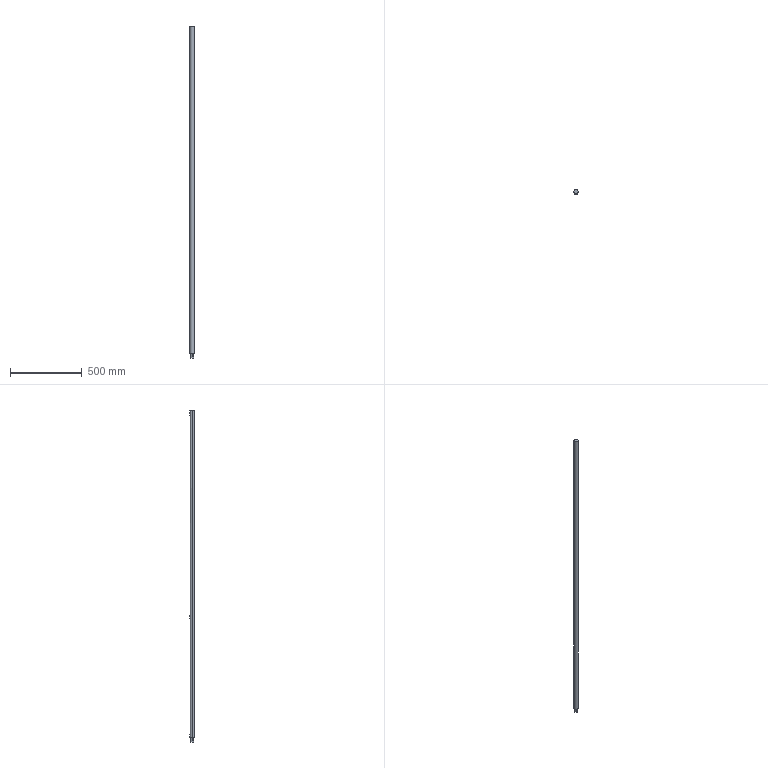Part | STEP file | Shaft dia30 2280V11 | 1 solid | 27 faces | box 30 x 30 x 2310 mm | volume 1619744 mm3 | plane 25 | cylinder 2 | commonest cylinder face diameters 30 x2